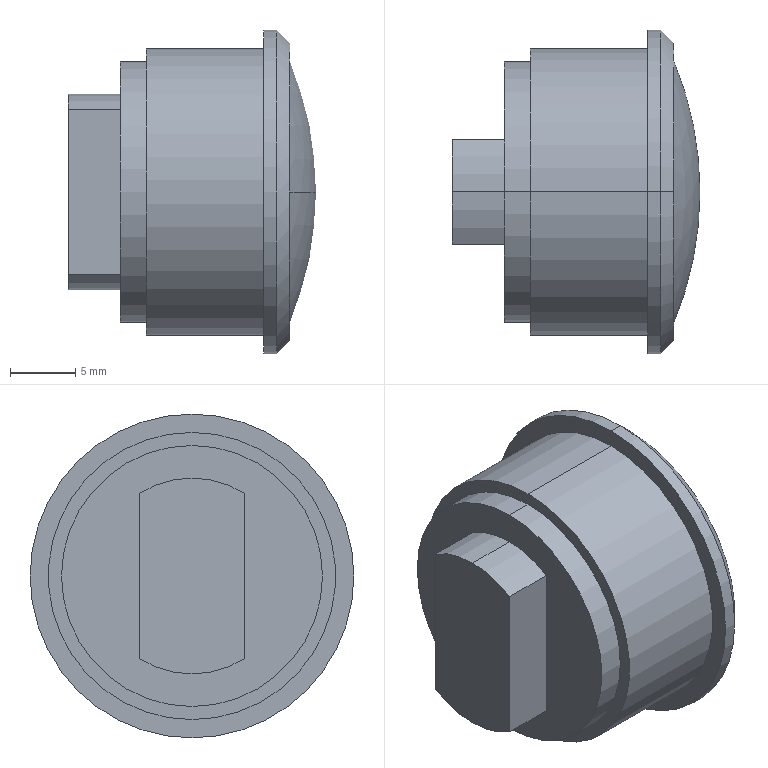Part | SolidWorks | features ICE 2, Revolution 2, Chamfer 1 | 1 solid | 25 faces | box 19 x 24.8 x 24.8 mm | volume 5733 mm3 | cylinder 13 | plane 8 | sphere 2 | cone 2 | commonest cylinder face diameters 20 x4 15 x3 20.2 x2 22 x2 24.8 x2
STEP:
#1=CARTESIAN_POINT('',(19.,0.,0.));
#2=VERTEX_POINT('',#1);
#3=CARTESIAN_POINT('',(17.,10.,0.));
#4=VERTEX_POINT('',#3);
#5=CARTESIAN_POINT('',(-7.,0.,0.));
#6=DIRECTION('',(0.,0.,1.));
#7=DIRECTION('',(1.,0.,0.));
#8=AXIS2_PLACEMENT_3D('',#5,#6,#7);
#9=CIRCLE('',#8,26.);
#10=EDGE_CURVE('',#2,#4,#9,.T.);
#11=ORIENTED_EDGE('',*,*,#10,.F.);
#12=CARTESIAN_POINT('',(17.,-10.,0.));
#13=VERTEX_POINT('',#12);
#14=CARTESIAN_POINT('',(-7.,0.,0.));
#15=DIRECTION('',(0.,0.,-1.));
#16=DIRECTION('',(0.,1.,0.));
#17=AXIS2_PLACEMENT_3D('',#14,#15,#16);
#18=CIRCLE('',#17,26.);
#19=EDGE_CURVE('',#2,#13,#18,.T.);
#20=ORIENTED_EDGE('',*,*,#19,.T.);
#21=CARTESIAN_POINT('',(17.,0.,-10.));
#22=VERTEX_POINT('',#21);
#23=CARTESIAN_POINT('',(17.,0.,0.));
#24=DIRECTION('',(1.,0.,0.));
#25=DIRECTION('',(0.,0.,-1.));
#26=AXIS2_PLACEMENT_3D('',#23,#24,#25);
#27=CIRCLE('',#26,10.);
#28=EDGE_CURVE('',#13,#22,#27,.T.);
#29=ORIENTED_EDGE('',*,*,#28,.T.);
#30=CARTESIAN_POINT('',(17.,0.,0.));
#31=DIRECTION('',(1.,0.,0.));
#32=DIRECTION('',(0.,0.,-1.));
#33=AXIS2_PLACEMENT_3D('',#30,#31,#32);
#34=CIRCLE('',#33,10.);
#35=EDGE_CURVE('',#22,#4,#34,.T.);
#36=ORIENTED_EDGE('',*,*,#35,.T.);
#37=EDGE_LOOP('',(#11,#20,#29,#36));
#38=FACE_OUTER_BOUND('',#37,.T.);
#39=CARTESIAN_POINT('',(-7.,0.,0.));
#40=DIRECTION('',(0.,0.,-1.));
#41=DIRECTION('',(0.,1.,0.));
#42=AXIS2_PLACEMENT_3D('',#39,#40,#41);
#43=SPHERICAL_SURFACE('',#42,26.);
#44=ADVANCED_FACE('',(#38),#43,.T.);
#45=CARTESIAN_POINT('',(14.,0.,-10.));
#46=VERTEX_POINT('',#45);
#47=CARTESIAN_POINT('',(14.,0.,10.));
#48=VERTEX_POINT('',#47);
#49=CARTESIAN_POINT('',(14.,0.,0.));
#50=DIRECTION('',(1.,0.,0.));
#51=DIRECTION('',(0.,0.,-1.));
#52=AXIS2_PLACEMENT_3D('',#49,#50,#51);
#53=CIRCLE('',#52,10.);
#54=EDGE_CURVE('',#46,#48,#53,.T.);
#55=ORIENTED_EDGE('',*,*,#54,.T.);
#56=CARTESIAN_POINT('',(17.,0.,10.));
#57=VERTEX_POINT('',#56);
#58=CARTESIAN_POINT('',(14.,0.,10.));
#59=DIRECTION('',(1.,0.,0.));
#60=VECTOR('',#59,1000.);
#61=LINE('',#58,#60);
#62=EDGE_CURVE('',#48,#57,#61,.T.);
#63=ORIENTED_EDGE('',*,*,#62,.T.);
#64=CARTESIAN_POINT('',(17.,0.,0.));
#65=DIRECTION('',(1.,0.,0.));
#66=DIRECTION('',(0.,0.,-1.));
#67=AXIS2_PLACEMENT_3D('',#64,#65,#66);
#68=CIRCLE('',#67,10.);
#69=EDGE_CURVE('',#4,#57,#68,.T.);
#70=ORIENTED_EDGE('',*,*,#69,.F.);
#71=ORIENTED_EDGE('',*,*,#35,.F.);
#72=CARTESIAN_POINT('',(14.,0.,-10.));
#73=DIRECTION('',(1.,0.,0.));
#74=VECTOR('',#73,1000.);
#75=LINE('',#72,#74);
#76=EDGE_CURVE('',#46,#22,#75,.T.);
#77=ORIENTED_EDGE('',*,*,#76,.F.);
#78=EDGE_LOOP('',(#55,#63,#70,#71,#77));
#79=FACE_OUTER_BOUND('',#78,.T.);
#80=CARTESIAN_POINT('',(14.,0.,0.));
#81=DIRECTION('',(1.,0.,0.));
#82=DIRECTION('',(0.,0.,-1.));
#83=AXIS2_PLACEMENT_3D('',#80,#81,#82);
#84=CYLINDRICAL_SURFACE('',#83,10.);
#85=ADVANCED_FACE('',(#79),#84,.T.);
#86=CARTESIAN_POINT('',(14.,0.,10.1));
#87=VERTEX_POINT('',#86);
#88=CARTESIAN_POINT('',(14.,0.,-10.1));
#89=VERTEX_POINT('',#88);
#90=CARTESIAN_POINT('',(14.,0.,0.));
#91=DIRECTION('',(1.,0.,0.));
#92=DIRECTION('',(0.,0.,-1.));
#93=AXIS2_PLACEMENT_3D('',#90,#91,#92);
#94=CIRCLE('',#93,10.1);
#95=EDGE_CURVE('',#87,#89,#94,.T.);
#96=ORIENTED_EDGE('',*,*,#95,.F.);
#97=CARTESIAN_POINT('',(17.,0.,10.1));
#98=VERTEX_POINT('',#97);
#99=CARTESIAN_POINT('',(14.,0.,10.1));
#100=DIRECTION('',(1.,0.,0.));
#101=VECTOR('',#100,1000.);
#102=LINE('',#99,#101);
#103=EDGE_CURVE('',#87,#98,#102,.T.);
#104=ORIENTED_EDGE('',*,*,#103,.T.);
#105=CARTESIAN_POINT('',(17.,0.,-10.1));
#106=VERTEX_POINT('',#105);
#107=CARTESIAN_POINT('',(17.,0.,0.));
#108=DIRECTION('',(1.,0.,0.));
#109=DIRECTION('',(0.,0.,-1.));
#110=AXIS2_PLACEMENT_3D('',#107,#108,#109);
#111=CIRCLE('',#110,10.1);
#112=EDGE_CURVE('',#98,#106,#111,.T.);
#113=ORIENTED_EDGE('',*,*,#112,.T.);
#114=CARTESIAN_POINT('',(14.,0.,-10.1));
#115=DIRECTION('',(1.,0.,0.));
#116=VECTOR('',#115,1000.);
#117=LINE('',#114,#116);
#118=EDGE_CURVE('',#89,#106,#117,.T.);
#119=ORIENTED_EDGE('',*,*,#118,.F.);
#120=EDGE_LOOP('',(#96,#104,#113,#119));
#121=FACE_OUTER_BOUND('',#120,.T.);
#122=CARTESIAN_POINT('',(14.,0.,0.));
#123=DIRECTION('',(1.,0.,0.));
#124=DIRECTION('',(0.,0.,-1.));
#125=AXIS2_PLACEMENT_3D('',#122,#123,#124);
#126=CYLINDRICAL_SURFACE('',#125,10.1);
#127=ADVANCED_FACE('',(#121),#126,.F.);
#128=CARTESIAN_POINT('',(17.,0.,-11.4));
#129=VERTEX_POINT('',#128);
#130=CARTESIAN_POINT('',(17.,0.,11.4));
#131=VERTEX_POINT('',#130);
#132=CARTESIAN_POINT('',(17.,0.,0.));
#133=DIRECTION('',(1.,0.,0.));
#134=DIRECTION('',(0.,0.,1.));
#135=AXIS2_PLACEMENT_3D('',#132,#133,#134);
#136=CIRCLE('',#135,11.4);
#137=EDGE_CURVE('',#129,#131,#136,.T.);
#138=ORIENTED_EDGE('',*,*,#137,.F.);
#139=CARTESIAN_POINT('',(16.,0.,-12.4));
#140=VERTEX_POINT('',#139);
#141=CARTESIAN_POINT('',(16.,0.,-12.4));
#142=DIRECTION('',(-0.7071,0.,-0.7071));
#143=VECTOR('',#142,1000.);
#144=LINE('',#141,#143);
#145=EDGE_CURVE('',#129,#140,#144,.T.);
#146=ORIENTED_EDGE('',*,*,#145,.T.);
#147=CARTESIAN_POINT('',(16.,0.,12.4));
#148=VERTEX_POINT('',#147);
#149=CARTESIAN_POINT('',(16.,0.,0.));
#150=DIRECTION('',(-1.,0.,0.));
#151=DIRECTION('',(0.,0.,1.));
#152=AXIS2_PLACEMENT_3D('',#149,#150,#151);
#153=CIRCLE('',#152,12.4);
#154=EDGE_CURVE('',#148,#140,#153,.T.);
#155=ORIENTED_EDGE('',*,*,#154,.F.);
#156=CARTESIAN_POINT('',(16.,0.,12.4));
#157=DIRECTION('',(-0.7071,0.,0.7071));
#158=VECTOR('',#157,1000.);
#159=LINE('',#156,#158);
#160=EDGE_CURVE('',#131,#148,#159,.T.);
#161=ORIENTED_EDGE('',*,*,#160,.F.);
#162=EDGE_LOOP('',(#138,#146,#155,#161));
#163=FACE_OUTER_BOUND('',#162,.T.);
#164=CARTESIAN_POINT('',(16.,0.,0.));
#165=DIRECTION('',(-1.,0.,0.));
#166=DIRECTION('',(0.,0.,1.));
#167=AXIS2_PLACEMENT_3D('',#164,#165,#166);
#168=CONICAL_SURFACE('',#167,12.4,0.7854);
#169=ADVANCED_FACE('',(#163),#168,.T.);
#170=CARTESIAN_POINT('',(6.,0.,10.));
#171=VERTEX_POINT('',#170);
#172=CARTESIAN_POINT('',(6.,0.,-10.));
#173=VERTEX_POINT('',#172);
#174=CARTESIAN_POINT('',(6.,0.,0.));
#175=DIRECTION('',(-1.,0.,0.));
#176=DIRECTION('',(0.,0.,1.));
#177=AXIS2_PLACEMENT_3D('',#174,#175,#176);
#178=CIRCLE('',#177,10.);
#179=EDGE_CURVE('',#171,#173,#178,.T.);
#180=ORIENTED_EDGE('',*,*,#179,.T.);
#181=CARTESIAN_POINT('',(4.,0.,-10.));
#182=VERTEX_POINT('',#181);
#183=CARTESIAN_POINT('',(0.,0.,-10.));
#184=DIRECTION('',(-1.,0.,0.));
#185=VECTOR('',#184,1000.);
#186=LINE('',#183,#185);
#187=EDGE_CURVE('',#173,#182,#186,.T.);
#188=ORIENTED_EDGE('',*,*,#187,.T.);
#189=CARTESIAN_POINT('',(4.,0.,10.));
#190=VERTEX_POINT('',#189);
#191=CARTESIAN_POINT('',(4.,0.,0.));
#192=DIRECTION('',(-1.,0.,0.));
#193=DIRECTION('',(0.,0.,1.));
#194=AXIS2_PLACEMENT_3D('',#191,#192,#193);
#195=CIRCLE('',#194,10.);
#196=EDGE_CURVE('',#190,#182,#195,.T.);
#197=ORIENTED_EDGE('',*,*,#196,.F.);
#198=CARTESIAN_POINT('',(0.,0.,10.));
#199=DIRECTION('',(-1.,0.,0.));
#200=VECTOR('',#199,1000.);
#201=LINE('',#198,#200);
#202=EDGE_CURVE('',#171,#190,#201,.T.);
#203=ORIENTED_EDGE('',*,*,#202,.F.);
#204=EDGE_LOOP('',(#180,#188,#197,#203));
#205=FACE_OUTER_BOUND('',#204,.T.);
#206=CARTESIAN_POINT('',(0.,0.,0.));
#207=DIRECTION('',(-1.,0.,0.));
#208=DIRECTION('',(0.,0.,1.));
#209=AXIS2_PLACEMENT_3D('',#206,#207,#208);
#210=CYLINDRICAL_SURFACE('',#209,10.);
#211=ADVANCED_FACE('',(#205),#210,.T.);
#212=CARTESIAN_POINT('',(15.,0.,11.));
#213=VERTEX_POINT('',#212);
#214=CARTESIAN_POINT('',(15.,0.,-11.));
#215=VERTEX_POINT('',#214);
#216=CARTESIAN_POINT('',(15.,0.,0.));
#217=DIRECTION('',(-1.,0.,0.));
#218=DIRECTION('',(0.,0.,1.));
#219=AXIS2_PLACEMENT_3D('',#216,#217,#218);
#220=CIRCLE('',#219,11.);
#221=EDGE_CURVE('',#213,#215,#220,.T.);
#222=ORIENTED_EDGE('',*,*,#221,.T.);
#223=CARTESIAN_POINT('',(6.,0.,-11.));
#224=VERTEX_POINT('',#223);
#225=CARTESIAN_POINT('',(0.,0.,-11.));
#226=DIRECTION('',(-1.,0.,0.));
#227=VECTOR('',#226,1000.);
#228=LINE('',#225,#227);
#229=EDGE_CURVE('',#215,#224,#228,.T.);
#230=ORIENTED_EDGE('',*,*,#229,.T.);
#231=CARTESIAN_POINT('',(6.,0.,11.));
#232=VERTEX_POINT('',#231);
#233=CARTESIAN_POINT('',(6.,0.,0.));
#234=DIRECTION('',(-1.,0.,0.));
#235=DIRECTION('',(0.,0.,1.));
#236=AXIS2_PLACEMENT_3D('',#233,#234,#235);
#237=CIRCLE('',#236,11.);
#238=EDGE_CURVE('',#232,#224,#237,.T.);
#239=ORIENTED_EDGE('',*,*,#238,.F.);
#240=CARTESIAN_POINT('',(0.,0.,11.));
#241=DIRECTION('',(-1.,0.,0.));
#242=VECTOR('',#241,1000.);
#243=LINE('',#240,#242);
#244=EDGE_CURVE('',#213,#232,#243,.T.);
#245=ORIENTED_EDGE('',*,*,#244,.F.);
#246=EDGE_LOOP('',(#222,#230,#239,#245));
#247=FACE_OUTER_BOUND('',#246,.T.);
#248=CARTESIAN_POINT('',(0.,0.,0.));
#249=DIRECTION('',(-1.,0.,0.));
#250=DIRECTION('',(0.,0.,1.));
#251=AXIS2_PLACEMENT_3D('',#248,#249,#250);
#252=CYLINDRICAL_SURFACE('',#251,11.);
#253=ADVANCED_FACE('',(#247),#252,.T.);
#254=ORIENTED_EDGE('',*,*,#154,.T.);
#255=CARTESIAN_POINT('',(15.,0.,-12.4));
#256=VERTEX_POINT('',#255);
#257=CARTESIAN_POINT('',(0.,0.,-12.4));
#258=DIRECTION('',(-1.,0.,0.));
#259=VECTOR('',#258,1000.);
#260=LINE('',#257,#259);
#261=EDGE_CURVE('',#140,#256,#260,.T.);
#262=ORIENTED_EDGE('',*,*,#261,.T.);
#263=CARTESIAN_POINT('',(15.,0.,12.4));
#264=VERTEX_POINT('',#263);
#265=CARTESIAN_POINT('',(15.,0.,0.));
#266=DIRECTION('',(-1.,0.,0.));
#267=DIRECTION('',(0.,0.,1.));
#268=AXIS2_PLACEMENT_3D('',#265,#266,#267);
#269=CIRCLE('',#268,12.4);
#270=EDGE_CURVE('',#264,#256,#269,.T.);
#271=ORIENTED_EDGE('',*,*,#270,.F.);
#272=CARTESIAN_POINT('',(0.,0.,12.4));
#273=DIRECTION('',(-1.,0.,0.));
#274=VECTOR('',#273,1000.);
#275=LINE('',#272,#274);
#276=EDGE_CURVE('',#148,#264,#275,.T.);
#277=ORIENTED_EDGE('',*,*,#276,.F.);
#278=EDGE_LOOP('',(#254,#262,#271,#277));
#279=FACE_OUTER_BOUND('',#278,.T.);
#280=CARTESIAN_POINT('',(0.,0.,0.));
#281=DIRECTION('',(-1.,0.,0.));
#282=DIRECTION('',(0.,0.,1.));
#283=AXIS2_PLACEMENT_3D('',#280,#281,#282);
#284=CYLINDRICAL_SURFACE('',#283,12.4);
#285=ADVANCED_FACE('',(#279),#284,.T.);
#286=CARTESIAN_POINT('',(4.,-4.,6.344));
#287=VERTEX_POINT('',#286);
#288=CARTESIAN_POINT('',(4.,0.,7.5));
#289=VERTEX_POINT('',#288);
#290=CARTESIAN_POINT('',(4.,0.,0.));
#291=DIRECTION('',(-1.,0.,0.));
#292=DIRECTION('',(0.,0.,1.));
#293=AXIS2_PLACEMENT_3D('',#290,#291,#292);
#294=CIRCLE('',#293,7.5);
#295=EDGE_CURVE('',#287,#289,#294,.T.);
#296=ORIENTED_EDGE('',*,*,#295,.T.);
#297=CARTESIAN_POINT('',(0.,0.,7.5));
#298=VERTEX_POINT('',#297);
#299=CARTESIAN_POINT('',(0.,0.,7.5));
#300=DIRECTION('',(-1.,0.,0.));
#301=VECTOR('',#300,1000.);
#302=LINE('',#299,#301);
#303=EDGE_CURVE('',#289,#298,#302,.T.);
#304=ORIENTED_EDGE('',*,*,#303,.T.);
#305=CARTESIAN_POINT('',(0.,-4.,6.344));
#306=VERTEX_POINT('',#305);
#307=CARTESIAN_POINT('',(0.,0.,0.));
#308=DIRECTION('',(-1.,0.,0.));
#309=DIRECTION('',(0.,0.,1.));
#310=AXIS2_PLACEMENT_3D('',#307,#308,#309);
#311=CIRCLE('',#310,7.5);
#312=EDGE_CURVE('',#306,#298,#311,.T.);
#313=ORIENTED_EDGE('',*,*,#312,.F.);
#314=CARTESIAN_POINT('',(0.,-4.,6.344));
#315=DIRECTION('',(-1.,0.,0.));
#316=VECTOR('',#315,1000.);
#317=LINE('',#314,#316);
#318=EDGE_CURVE('',#287,#306,#317,.T.);
#319=ORIENTED_EDGE('',*,*,#318,.F.);
#320=EDGE_LOOP('',(#296,#304,#313,#319));
#321=FACE_OUTER_BOUND('',#320,.T.);
#322=CARTESIAN_POINT('',(0.,0.,0.));
#323=DIRECTION('',(-1.,0.,0.));
#324=DIRECTION('',(0.,0.,1.));
#325=AXIS2_PLACEMENT_3D('',#322,#323,#324);
#326=CYLINDRICAL_SURFACE('',#325,7.5);
#327=ADVANCED_FACE('',(#321),#326,.T.);
#328=CARTESIAN_POINT('',(0.,-4.,-6.344));
#329=VERTEX_POINT('',#328);
#330=CARTESIAN_POINT('',(0.,-4.,-8.401));
#331=DIRECTION('',(0.,0.,1.));
#332=VECTOR('',#331,1000.);
#333=LINE('',#330,#332);
#334=EDGE_CURVE('',#329,#306,#333,.T.);
#335=ORIENTED_EDGE('',*,*,#334,.T.);
#336=ORIENTED_EDGE('',*,*,#312,.T.);
#337=CARTESIAN_POINT('',(0.,4.,6.344));
#338=VERTEX_POINT('',#337);
#339=CARTESIAN_POINT('',(0.,0.,0.));
#340=DIRECTION('',(-1.,0.,0.));
#341=DIRECTION('',(0.,0.,1.));
#342=AXIS2_PLACEMENT_3D('',#339,#340,#341);
#343=CIRCLE('',#342,7.5);
#344=EDGE_CURVE('',#298,#338,#343,.T.);
#345=ORIENTED_EDGE('',*,*,#344,.T.);
#346=CARTESIAN_POINT('',(0.,4.,-6.344));
#347=VERTEX_POINT('',#346);
#348=CARTESIAN_POINT('',(0.,4.,-8.401));
#349=DIRECTION('',(0.,0.,-1.));
#350=VECTOR('',#349,1000.);
#351=LINE('',#348,#350);
#352=EDGE_CURVE('',#338,#347,#351,.T.);
#353=ORIENTED_EDGE('',*,*,#352,.T.);
#354=CARTESIAN_POINT('',(0.,0.,0.));
#355=DIRECTION('',(-1.,0.,0.));
#356=DIRECTION('',(0.,0.,1.));
#357=AXIS2_PLACEMENT_3D('',#354,#355,#356);
#358=CIRCLE('',#357,7.5);
#359=EDGE_CURVE('',#347,#329,#358,.T.);
#360=ORIENTED_EDGE('',*,*,#359,.T.);
#361=EDGE_LOOP('',(#335,#336,#345,#353,#360));
#362=FACE_OUTER_BOUND('',#361,.T.);
#363=CARTESIAN_POINT('',(0.,0.,-7.5));
#364=DIRECTION('',(1.,0.,0.));
#365=DIRECTION('',(0.,0.,-1.));
#366=AXIS2_PLACEMENT_3D('',#363,#364,#365);
#367=PLANE('',#366);
#368=ADVANCED_FACE('',(#362),#367,.F.);
#369=ORIENTED_EDGE('',*,*,#303,.F.);
#370=CARTESIAN_POINT('',(4.,4.,6.344));
#371=VERTEX_POINT('',#370);
#372=CARTESIAN_POINT('',(4.,0.,0.));
#373=DIRECTION('',(-1.,0.,0.));
#374=DIRECTION('',(0.,0.,1.));
#375=AXIS2_PLACEMENT_3D('',#372,#373,#374);
#376=CIRCLE('',#375,7.5);
#377=EDGE_CURVE('',#289,#371,#376,.T.);
#378=ORIENTED_EDGE('',*,*,#377,.T.);
#379=CARTESIAN_POINT('',(0.,4.,6.344));
#380=DIRECTION('',(1.,0.,0.));
#381=VECTOR('',#380,1000.);
#382=LINE('',#379,#381);
#383=EDGE_CURVE('',#338,#371,#382,.T.);
#384=ORIENTED_EDGE('',*,*,#383,.F.);
#385=ORIENTED_EDGE('',*,*,#344,.F.);
#386=EDGE_LOOP('',(#369,#378,#384,#385));
#387=FACE_OUTER_BOUND('',#386,.T.);
#388=CARTESIAN_POINT('',(0.,0.,0.));
#389=DIRECTION('',(-1.,0.,0.));
#390=DIRECTION('',(0.,0.,1.));
#391=AXIS2_PLACEMENT_3D('',#388,#389,#390);
#392=CYLINDRICAL_SURFACE('',#391,7.5);
#393=ADVANCED_FACE('',(#387),#392,.T.);
#394=CARTESIAN_POINT('',(4.,-4.,-6.344));
#395=VERTEX_POINT('',#394);
#396=CARTESIAN_POINT('',(0.,-4.,-6.344));
#397=DIRECTION('',(1.,0.,0.));
#398=VECTOR('',#397,1000.);
#399=LINE('',#396,#398);
#400=EDGE_CURVE('',#329,#395,#399,.T.);
#401=ORIENTED_EDGE('',*,*,#400,.F.);
#402=ORIENTED_EDGE('',*,*,#359,.F.);
#403=CARTESIAN_POINT('',(4.,4.,-6.344));
#404=VERTEX_POINT('',#403);
#405=CARTESIAN_POINT('',(0.,4.,-6.344));
#406=DIRECTION('',(-1.,0.,0.));
#407=VECTOR('',#406,1000.);
#408=LINE('',#405,#407);
#409=EDGE_CURVE('',#404,#347,#408,.T.);
#410=ORIENTED_EDGE('',*,*,#409,.F.);
#411=CARTESIAN_POINT('',(4.,0.,0.));
#412=DIRECTION('',(-1.,0.,0.));
#413=DIRECTION('',(0.,0.,1.));
#414=AXIS2_PLACEMENT_3D('',#411,#412,#413);
#415=CIRCLE('',#414,7.5);
#416=EDGE_CURVE('',#404,#395,#415,.T.);
#417=ORIENTED_EDGE('',*,*,#416,.T.);
#418=EDGE_LOOP('',(#401,#402,#410,#417));
#419=FACE_OUTER_BOUND('',#418,.T.);
#420=CARTESIAN_POINT('',(0.,0.,0.));
#421=DIRECTION('',(-1.,0.,0.));
#422=DIRECTION('',(0.,0.,1.));
#423=AXIS2_PLACEMENT_3D('',#420,#421,#422);
#424=CYLINDRICAL_SURFACE('',#423,7.5);
#425=ADVANCED_FACE('',(#419),#424,.T.);
#426=CARTESIAN_POINT('',(17.,0.,0.));
#427=DIRECTION('',(1.,0.,0.));
#428=DIRECTION('',(0.,0.,-1.));
#429=AXIS2_PLACEMENT_3D('',#426,#427,#428);
#430=CIRCLE('',#429,10.1);
#431=EDGE_CURVE('',#106,#98,#430,.T.);
#432=ORIENTED_EDGE('',*,*,#431,.F.);
#433=ORIENTED_EDGE('',*,*,#112,.F.);
#434=EDGE_LOOP('',(#432,#433));
#435=FACE_BOUND('',#434,.T.);
#436=CARTESIAN_POINT('',(17.,0.,0.));
#437=DIRECTION('',(1.,0.,0.));
#438=DIRECTION('',(0.,0.,1.));
#439=AXIS2_PLACEMENT_3D('',#436,#437,#438);
#440=CIRCLE('',#439,11.4);
#441=EDGE_CURVE('',#131,#129,#440,.T.);
#442=ORIENTED_EDGE('',*,*,#441,.T.);
#443=ORIENTED_EDGE('',*,*,#137,.T.);
#444=EDGE_LOOP('',(#442,#443));
#445=FACE_OUTER_BOUND('',#444,.T.);
#446=CARTESIAN_POINT('',(17.,0.,0.));
#447=DIRECTION('',(-1.,0.,0.));
#448=DIRECTION('',(0.,0.,1.));
#449=AXIS2_PLACEMENT_3D('',#446,#447,#448);
#450=PLANE('',#449);
#451=ADVANCED_FACE('',(#435,#445),#450,.F.);
#452=ORIENTED_EDGE('',*,*,#261,.F.);
#453=CARTESIAN_POINT('',(16.,0.,0.));
#454=DIRECTION('',(-1.,0.,0.));
#455=DIRECTION('',(0.,0.,1.));
#456=AXIS2_PLACEMENT_3D('',#453,#454,#455);
#457=CIRCLE('',#456,12.4);
#458=EDGE_CURVE('',#140,#148,#457,.T.);
#459=ORIENTED_EDGE('',*,*,#458,.T.);
#460=ORIENTED_EDGE('',*,*,#276,.T.);
#461=CARTESIAN_POINT('',(15.,0.,0.));
#462=DIRECTION('',(-1.,0.,0.));
#463=DIRECTION('',(0.,0.,1.));
#464=AXIS2_PLACEMENT_3D('',#461,#462,#463);
#465=CIRCLE('',#464,12.4);
#466=EDGE_CURVE('',#256,#264,#465,.T.);
#467=ORIENTED_EDGE('',*,*,#466,.F.);
#468=EDGE_LOOP('',(#452,#459,#460,#467));
#469=FACE_OUTER_BOUND('',#468,.T.);
#470=CARTESIAN_POINT('',(0.,0.,0.));
#471=DIRECTION('',(-1.,0.,0.));
#472=DIRECTION('',(0.,0.,1.));
#473=AXIS2_PLACEMENT_3D('',#470,#471,#472);
#474=CYLINDRICAL_SURFACE('',#473,12.4);
#475=ADVANCED_FACE('',(#469),#474,.T.);
#476=ORIENTED_EDGE('',*,*,#221,.F.);
#477=CARTESIAN_POINT('',(15.,0.,0.));
#478=DIRECTION('',(-1.,0.,0.));
#479=DIRECTION('',(0.,0.,1.));
#480=AXIS2_PLACEMENT_3D('',#477,#478,#479);
#481=CIRCLE('',#480,11.);
#482=EDGE_CURVE('',#215,#213,#481,.T.);
#483=ORIENTED_EDGE('',*,*,#482,.F.);
#484=EDGE_LOOP('',(#476,#483));
#485=FACE_BOUND('',#484,.T.);
#486=ORIENTED_EDGE('',*,*,#270,.T.);
#487=ORIENTED_EDGE('',*,*,#466,.T.);
#488=EDGE_LOOP('',(#486,#487));
#489=FACE_OUTER_BOUND('',#488,.T.);
#490=CARTESIAN_POINT('',(15.,0.,-12.4));
#491=DIRECTION('',(1.,0.,0.));
#492=DIRECTION('',(0.,0.,-1.));
#493=AXIS2_PLACEMENT_3D('',#490,#491,#492);
#494=PLANE('',#493);
#495=ADVANCED_FACE('',(#485,#489),#494,.F.);
#496=ORIENTED_EDGE('',*,*,#229,.F.);
#497=ORIENTED_EDGE('',*,*,#482,.T.);
#498=ORIENTED_EDGE('',*,*,#244,.T.);
#499=CARTESIAN_POINT('',(6.,0.,0.));
#500=DIRECTION('',(-1.,0.,0.));
#501=DIRECTION('',(0.,0.,1.));
#502=AXIS2_PLACEMENT_3D('',#499,#500,#501);
#503=CIRCLE('',#502,11.);
#504=EDGE_CURVE('',#224,#232,#503,.T.);
#505=ORIENTED_EDGE('',*,*,#504,.F.);
#506=EDGE_LOOP('',(#496,#497,#498,#505));
#507=FACE_OUTER_BOUND('',#506,.T.);
#508=CARTESIAN_POINT('',(0.,0.,0.));
#509=DIRECTION('',(-1.,0.,0.));
#510=DIRECTION('',(0.,0.,1.));
#511=AXIS2_PLACEMENT_3D('',#508,#509,#510);
#512=CYLINDRICAL_SURFACE('',#511,11.);
#513=ADVANCED_FACE('',(#507),#512,.T.);
#514=ORIENTED_EDGE('',*,*,#179,.F.);
#515=CARTESIAN_POINT('',(6.,0.,0.));
#516=DIRECTION('',(-1.,0.,0.));
#517=DIRECTION('',(0.,0.,1.));
#518=AXIS2_PLACEMENT_3D('',#515,#516,#517);
#519=CIRCLE('',#518,10.);
#520=EDGE_CURVE('',#173,#171,#519,.T.);
#521=ORIENTED_EDGE('',*,*,#520,.F.);
#522=EDGE_LOOP('',(#514,#521));
#523=FACE_BOUND('',#522,.T.);
#524=ORIENTED_EDGE('',*,*,#238,.T.);
#525=ORIENTED_EDGE('',*,*,#504,.T.);
#526=EDGE_LOOP('',(#524,#525));
#527=FACE_OUTER_BOUND('',#526,.T.);
#528=CARTESIAN_POINT('',(6.,0.,-11.));
#529=DIRECTION('',(1.,0.,0.));
#530=DIRECTION('',(0.,0.,-1.));
#531=AXIS2_PLACEMENT_3D('',#528,#529,#530);
#532=PLANE('',#531);
#533=ADVANCED_FACE('',(#523,#527),#532,.F.);
#534=ORIENTED_EDGE('',*,*,#187,.F.);
#535=ORIENTED_EDGE('',*,*,#520,.T.);
#536=ORIENTED_EDGE('',*,*,#202,.T.);
#537=CARTESIAN_POINT('',(4.,0.,0.));
#538=DIRECTION('',(-1.,0.,0.));
#539=DIRECTION('',(0.,0.,1.));
#540=AXIS2_PLACEMENT_3D('',#537,#538,#539);
#541=CIRCLE('',#540,10.);
#542=EDGE_CURVE('',#182,#190,#541,.T.);
#543=ORIENTED_EDGE('',*,*,#542,.F.);
#544=EDGE_LOOP('',(#534,#535,#536,#543));
#545=FACE_OUTER_BOUND('',#544,.T.);
#546=CARTESIAN_POINT('',(0.,0.,0.));
#547=DIRECTION('',(-1.,0.,0.));
#548=DIRECTION('',(0.,0.,1.));
#549=AXIS2_PLACEMENT_3D('',#546,#547,#548);
#550=CYLINDRICAL_SURFACE('',#549,10.);
#551=ADVANCED_FACE('',(#545),#550,.T.);
#552=ORIENTED_EDGE('',*,*,#295,.F.);
#553=CARTESIAN_POINT('',(4.,-4.,-8.401));
#554=DIRECTION('',(0.,0.,1.));
#555=VECTOR('',#554,1000.);
#556=LINE('',#553,#555);
#557=EDGE_CURVE('',#395,#287,#556,.T.);
#558=ORIENTED_EDGE('',*,*,#557,.F.);
#559=ORIENTED_EDGE('',*,*,#416,.F.);
#560=CARTESIAN_POINT('',(4.,4.,-8.401));
#561=DIRECTION('',(0.,0.,-1.));
#562=VECTOR('',#561,1000.);
#563=LINE('',#560,#562);
#564=EDGE_CURVE('',#371,#404,#563,.T.);
#565=ORIENTED_EDGE('',*,*,#564,.F.);
#566=ORIENTED_EDGE('',*,*,#377,.F.);
#567=EDGE_LOOP('',(#552,#558,#559,#565,#566));
#568=FACE_BOUND('',#567,.T.);
#569=ORIENTED_EDGE('',*,*,#196,.T.);
#570=ORIENTED_EDGE('',*,*,#542,.T.);
#571=EDGE_LOOP('',(#569,#570));
#572=FACE_OUTER_BOUND('',#571,.T.);
#573=CARTESIAN_POINT('',(4.,0.,-10.));
#574=DIRECTION('',(1.,0.,0.));
#575=DIRECTION('',(0.,0.,-1.));
#576=AXIS2_PLACEMENT_3D('',#573,#574,#575);
#577=PLANE('',#576);
#578=ADVANCED_FACE('',(#568,#572),#577,.F.);
#579=ORIENTED_EDGE('',*,*,#145,.F.);
#580=ORIENTED_EDGE('',*,*,#441,.F.);
#581=ORIENTED_EDGE('',*,*,#160,.T.);
#582=ORIENTED_EDGE('',*,*,#458,.F.);
#583=EDGE_LOOP('',(#579,#580,#581,#582));
#584=FACE_OUTER_BOUND('',#583,.T.);
#585=CARTESIAN_POINT('',(16.,0.,0.));
#586=DIRECTION('',(-1.,0.,0.));
#587=DIRECTION('',(0.,0.,1.));
#588=AXIS2_PLACEMENT_3D('',#585,#586,#587);
#589=CONICAL_SURFACE('',#588,12.4,0.7854);
#590=ADVANCED_FACE('',(#584),#589,.T.);
#591=ORIENTED_EDGE('',*,*,#318,.T.);
#592=ORIENTED_EDGE('',*,*,#334,.F.);
#593=ORIENTED_EDGE('',*,*,#400,.T.);
#594=ORIENTED_EDGE('',*,*,#557,.T.);
#595=EDGE_LOOP('',(#591,#592,#593,#594));
#596=FACE_OUTER_BOUND('',#595,.T.);
#597=CARTESIAN_POINT('',(39.423,-4.,-8.401));
#598=DIRECTION('',(0.,-1.,0.));
#599=DIRECTION('',(0.,0.,-1.));
#600=AXIS2_PLACEMENT_3D('',#597,#598,#599);
#601=PLANE('',#600);
#602=ADVANCED_FACE('',(#596),#601,.T.);
#603=ORIENTED_EDGE('',*,*,#409,.T.);
#604=ORIENTED_EDGE('',*,*,#352,.F.);
#605=ORIENTED_EDGE('',*,*,#383,.T.);
#606=ORIENTED_EDGE('',*,*,#564,.T.);
#607=EDGE_LOOP('',(#603,#604,#605,#606));
#608=FACE_OUTER_BOUND('',#607,.T.);
#609=CARTESIAN_POINT('',(39.423,4.,-8.401));
#610=DIRECTION('',(0.,1.,0.));
#611=DIRECTION('',(0.,0.,1.));
#612=AXIS2_PLACEMENT_3D('',#609,#610,#611);
#613=PLANE('',#612);
#614=ADVANCED_FACE('',(#608),#613,.T.);
#615=ORIENTED_EDGE('',*,*,#103,.F.);
#616=CARTESIAN_POINT('',(14.,0.,0.));
#617=DIRECTION('',(1.,0.,0.));
#618=DIRECTION('',(0.,0.,-1.));
#619=AXIS2_PLACEMENT_3D('',#616,#617,#618);
#620=CIRCLE('',#619,10.1);
#621=EDGE_CURVE('',#89,#87,#620,.T.);
#622=ORIENTED_EDGE('',*,*,#621,.F.);
#623=ORIENTED_EDGE('',*,*,#118,.T.);
#624=ORIENTED_EDGE('',*,*,#431,.T.);
#625=EDGE_LOOP('',(#615,#622,#623,#624));
#626=FACE_OUTER_BOUND('',#625,.T.);
#627=CARTESIAN_POINT('',(14.,0.,0.));
#628=DIRECTION('',(1.,0.,0.));
#629=DIRECTION('',(0.,0.,-1.));
#630=AXIS2_PLACEMENT_3D('',#627,#628,#629);
#631=CYLINDRICAL_SURFACE('',#630,10.1);
#632=ADVANCED_FACE('',(#626),#631,.F.);
#633=ORIENTED_EDGE('',*,*,#54,.F.);
#634=CARTESIAN_POINT('',(14.,0.,0.));
#635=DIRECTION('',(1.,0.,0.));
#636=DIRECTION('',(0.,0.,-1.));
#637=AXIS2_PLACEMENT_3D('',#634,#635,#636);
#638=CIRCLE('',#637,10.);
#639=EDGE_CURVE('',#48,#46,#638,.T.);
#640=ORIENTED_EDGE('',*,*,#639,.F.);
#641=EDGE_LOOP('',(#633,#640));
#642=FACE_BOUND('',#641,.T.);
#643=ORIENTED_EDGE('',*,*,#621,.T.);
#644=ORIENTED_EDGE('',*,*,#95,.T.);
#645=EDGE_LOOP('',(#643,#644));
#646=FACE_OUTER_BOUND('',#645,.T.);
#647=CARTESIAN_POINT('',(14.,0.,0.));
#648=DIRECTION('',(1.,0.,0.));
#649=DIRECTION('',(0.,0.,-1.));
#650=AXIS2_PLACEMENT_3D('',#647,#648,#649);
#651=PLANE('',#650);
#652=ADVANCED_FACE('',(#642,#646),#651,.T.);
#653=ORIENTED_EDGE('',*,*,#62,.F.);
#654=ORIENTED_EDGE('',*,*,#639,.T.);
#655=ORIENTED_EDGE('',*,*,#76,.T.);
#656=ORIENTED_EDGE('',*,*,#28,.F.);
#657=CARTESIAN_POINT('',(17.,0.,0.));
#658=DIRECTION('',(1.,0.,0.));
#659=DIRECTION('',(0.,0.,-1.));
#660=AXIS2_PLACEMENT_3D('',#657,#658,#659);
#661=CIRCLE('',#660,10.);
#662=EDGE_CURVE('',#57,#13,#661,.T.);
#663=ORIENTED_EDGE('',*,*,#662,.F.);
#664=EDGE_LOOP('',(#653,#654,#655,#656,#663));
#665=FACE_OUTER_BOUND('',#664,.T.);
#666=CARTESIAN_POINT('',(14.,0.,0.));
#667=DIRECTION('',(1.,0.,0.));
#668=DIRECTION('',(0.,0.,-1.));
#669=AXIS2_PLACEMENT_3D('',#666,#667,#668);
#670=CYLINDRICAL_SURFACE('',#669,10.);
#671=ADVANCED_FACE('',(#665),#670,.T.);
#672=ORIENTED_EDGE('',*,*,#19,.F.);
#673=ORIENTED_EDGE('',*,*,#10,.T.);
#674=ORIENTED_EDGE('',*,*,#69,.T.);
#675=ORIENTED_EDGE('',*,*,#662,.T.);
#676=EDGE_LOOP('',(#672,#673,#674,#675));
#677=FACE_OUTER_BOUND('',#676,.T.);
#678=CARTESIAN_POINT('',(-7.,0.,0.));
#679=DIRECTION('',(0.,0.,-1.));
#680=DIRECTION('',(0.,1.,0.));
#681=AXIS2_PLACEMENT_3D('',#678,#679,#680);
#682=SPHERICAL_SURFACE('',#681,26.);
#683=ADVANCED_FACE('',(#677),#682,.T.);
#684=CLOSED_SHELL('',(#44,#85,#127,#169,#211,#253,#285,#327,#368,#393,#425,#451,#475,#495,#513,#533,#551,#578,#590,#602,#614,#632,#652,#671,#683));
#685=MANIFOLD_SOLID_BREP('',#684);
#686=CARTESIAN_POINT('',(0.,0.,0.));
#687=DIRECTION('',(0.,0.,1.));
#688=DIRECTION('',(1.,0.,0.));
#689=AXIS2_PLACEMENT_3D('',#686,#687,#688);
#690=(LENGTH_UNIT()NAMED_UNIT(*)SI_UNIT(.MILLI.,.METRE.));
#691=UNCERTAINTY_MEASURE_WITH_UNIT(LENGTH_MEASURE(0.00001),#690,'','');
#692=(NAMED_UNIT(*)PLANE_ANGLE_UNIT()SI_UNIT($,.RADIAN.));
#693=(NAMED_UNIT(*)SI_UNIT($,.STERADIAN.)SOLID_ANGLE_UNIT());
#694=(GEOMETRIC_REPRESENTATION_CONTEXT(3)GLOBAL_UNCERTAINTY_ASSIGNED_CONTEXT((#691))GLOBAL_UNIT_ASSIGNED_CONTEXT((#690,#692,#693))REPRESENTATION_CONTEXT('',''));
#695=ADVANCED_BREP_SHAPE_REPRESENTATION('',(#685,#689),#694);